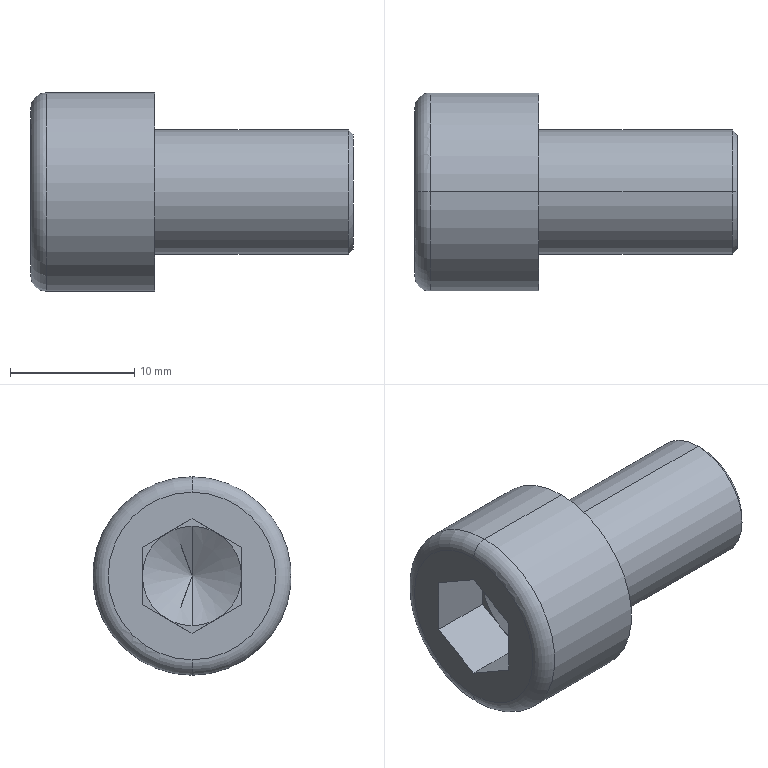Part | SolidWorks | features Fillet 2, RevCut 2, Boss 1, Chamfer 1, Cut 1, Extrusion 1, LPattern 1 | 1 solid | 25 faces | box 26 x 16 x 16 mm | volume 2933 mm3 | plane 15 | cone 4 | cylinder 4 | torus 2 | commonest cylinder face diameters 10 x2 16 x2
STEP:
#1=CARTESIAN_POINT('',(26.,0.,-4.6));
#2=VERTEX_POINT('',#1);
#3=CARTESIAN_POINT('',(26.,0.,4.6));
#4=VERTEX_POINT('',#3);
#5=CARTESIAN_POINT('',(26.,0.,0.));
#6=DIRECTION('',(1.,0.,0.));
#7=DIRECTION('',(0.,0.,-1.));
#8=AXIS2_PLACEMENT_3D('',#5,#6,#7);
#9=CIRCLE('',#8,4.6);
#10=EDGE_CURVE('',#2,#4,#9,.T.);
#11=ORIENTED_EDGE('',*,*,#10,.F.);
#12=CARTESIAN_POINT('',(25.6,0.,-5.));
#13=VERTEX_POINT('',#12);
#14=CARTESIAN_POINT('',(26.,0.,-4.6));
#15=DIRECTION('',(-0.7071,0.,-0.7071));
#16=VECTOR('',#15,1000.);
#17=LINE('',#14,#16);
#18=EDGE_CURVE('',#2,#13,#17,.T.);
#19=ORIENTED_EDGE('',*,*,#18,.T.);
#20=CARTESIAN_POINT('',(25.6,0.,5.));
#21=VERTEX_POINT('',#20);
#22=CARTESIAN_POINT('',(25.6,0.,0.));
#23=DIRECTION('',(-1.,0.,0.));
#24=DIRECTION('',(0.,0.,-1.));
#25=AXIS2_PLACEMENT_3D('',#22,#23,#24);
#26=CIRCLE('',#25,5.);
#27=EDGE_CURVE('',#21,#13,#26,.T.);
#28=ORIENTED_EDGE('',*,*,#27,.F.);
#29=CARTESIAN_POINT('',(26.,0.,4.6));
#30=DIRECTION('',(-0.7071,0.,0.7071));
#31=VECTOR('',#30,1000.);
#32=LINE('',#29,#31);
#33=EDGE_CURVE('',#4,#21,#32,.T.);
#34=ORIENTED_EDGE('',*,*,#33,.F.);
#35=EDGE_LOOP('',(#11,#19,#28,#34));
#36=FACE_OUTER_BOUND('',#35,.T.);
#37=CARTESIAN_POINT('',(26.,0.,0.));
#38=DIRECTION('',(-1.,0.,0.));
#39=DIRECTION('',(0.,0.,1.));
#40=AXIS2_PLACEMENT_3D('',#37,#38,#39);
#41=CONICAL_SURFACE('',#40,4.6,0.7854);
#42=ADVANCED_FACE('',(#36),#41,.T.);
#43=CARTESIAN_POINT('',(0.,0.,6.75));
#44=VERTEX_POINT('',#43);
#45=CARTESIAN_POINT('',(0.,0.,-6.75));
#46=VERTEX_POINT('',#45);
#47=CARTESIAN_POINT('',(0.,0.,0.));
#48=DIRECTION('',(-1.,0.,0.));
#49=DIRECTION('',(0.,0.,-1.));
#50=AXIS2_PLACEMENT_3D('',#47,#48,#49);
#51=CIRCLE('',#50,6.75);
#52=EDGE_CURVE('',#44,#46,#51,.T.);
#53=ORIENTED_EDGE('',*,*,#52,.F.);
#54=CARTESIAN_POINT('',(1.25,0.,8.));
#55=VERTEX_POINT('',#54);
#56=CARTESIAN_POINT('',(1.25,0.,6.75));
#57=DIRECTION('',(0.,1.,0.));
#58=DIRECTION('',(0.,0.,1.));
#59=AXIS2_PLACEMENT_3D('',#56,#57,#58);
#60=CIRCLE('',#59,1.25);
#61=EDGE_CURVE('',#44,#55,#60,.T.);
#62=ORIENTED_EDGE('',*,*,#61,.T.);
#63=CARTESIAN_POINT('',(1.25,0.,-8.));
#64=VERTEX_POINT('',#63);
#65=CARTESIAN_POINT('',(1.25,0.,0.));
#66=DIRECTION('',(1.,0.,0.));
#67=DIRECTION('',(0.,0.,-1.));
#68=AXIS2_PLACEMENT_3D('',#65,#66,#67);
#69=CIRCLE('',#68,8.);
#70=EDGE_CURVE('',#64,#55,#69,.T.);
#71=ORIENTED_EDGE('',*,*,#70,.F.);
#72=CARTESIAN_POINT('',(1.25,0.,-6.75));
#73=DIRECTION('',(0.,-1.,0.));
#74=DIRECTION('',(0.,0.,-1.));
#75=AXIS2_PLACEMENT_3D('',#72,#73,#74);
#76=CIRCLE('',#75,1.25);
#77=EDGE_CURVE('',#46,#64,#76,.T.);
#78=ORIENTED_EDGE('',*,*,#77,.F.);
#79=EDGE_LOOP('',(#53,#62,#71,#78));
#80=FACE_OUTER_BOUND('',#79,.T.);
#81=CARTESIAN_POINT('',(1.25,0.,0.));
#82=DIRECTION('',(1.,0.,0.));
#83=DIRECTION('',(0.,0.,-1.));
#84=AXIS2_PLACEMENT_3D('',#81,#82,#83);
#85=TOROIDAL_SURFACE('',#84,6.75,1.25);
#86=ADVANCED_FACE('',(#80),#85,.T.);
#87=CARTESIAN_POINT('',(7.309,0.,0.));
#88=VERTEX_POINT('',#87);
#89=CARTESIAN_POINT('',(5.,0.,4.));
#90=VERTEX_POINT('',#89);
#91=CARTESIAN_POINT('',(5.,0.,4.));
#92=DIRECTION('',(-0.5,0.,0.866));
#93=VECTOR('',#92,1000.);
#94=LINE('',#91,#93);
#95=EDGE_CURVE('',#88,#90,#94,.T.);
#96=ORIENTED_EDGE('',*,*,#95,.F.);
#97=CARTESIAN_POINT('',(5.,0.,-4.));
#98=VERTEX_POINT('',#97);
#99=CARTESIAN_POINT('',(5.,0.,-4.));
#100=DIRECTION('',(-0.5,0.,-0.866));
#101=VECTOR('',#100,1000.);
#102=LINE('',#99,#101);
#103=EDGE_CURVE('',#88,#98,#102,.T.);
#104=ORIENTED_EDGE('',*,*,#103,.T.);
#105=CARTESIAN_POINT('',(5.,-2.,-3.464));
#106=VERTEX_POINT('',#105);
#107=CARTESIAN_POINT('',(5.,0.,0.));
#108=DIRECTION('',(-1.,0.,0.));
#109=DIRECTION('',(0.,0.,-1.));
#110=AXIS2_PLACEMENT_3D('',#107,#108,#109);
#111=CIRCLE('',#110,4.);
#112=EDGE_CURVE('',#98,#106,#111,.T.);
#113=ORIENTED_EDGE('',*,*,#112,.T.);
#114=CARTESIAN_POINT('',(5.,-4.,0.));
#115=VERTEX_POINT('',#114);
#116=CARTESIAN_POINT('',(5.,0.,0.));
#117=DIRECTION('',(-1.,0.,0.));
#118=DIRECTION('',(0.,0.,-1.));
#119=AXIS2_PLACEMENT_3D('',#116,#117,#118);
#120=CIRCLE('',#119,4.);
#121=EDGE_CURVE('',#106,#115,#120,.T.);
#122=ORIENTED_EDGE('',*,*,#121,.T.);
#123=CARTESIAN_POINT('',(5.,-2.,3.464));
#124=VERTEX_POINT('',#123);
#125=CARTESIAN_POINT('',(5.,0.,0.));
#126=DIRECTION('',(-1.,0.,0.));
#127=DIRECTION('',(0.,0.,-1.));
#128=AXIS2_PLACEMENT_3D('',#125,#126,#127);
#129=CIRCLE('',#128,4.);
#130=EDGE_CURVE('',#115,#124,#129,.T.);
#131=ORIENTED_EDGE('',*,*,#130,.T.);
#132=CARTESIAN_POINT('',(5.,0.,0.));
#133=DIRECTION('',(-1.,0.,0.));
#134=DIRECTION('',(0.,0.,-1.));
#135=AXIS2_PLACEMENT_3D('',#132,#133,#134);
#136=CIRCLE('',#135,4.);
#137=EDGE_CURVE('',#124,#90,#136,.T.);
#138=ORIENTED_EDGE('',*,*,#137,.T.);
#139=EDGE_LOOP('',(#96,#104,#113,#122,#131,#138));
#140=FACE_OUTER_BOUND('',#139,.T.);
#141=CARTESIAN_POINT('',(5.,0.,0.));
#142=DIRECTION('',(-1.,0.,0.));
#143=DIRECTION('',(0.,0.,1.));
#144=AXIS2_PLACEMENT_3D('',#141,#142,#143);
#145=CONICAL_SURFACE('',#144,4.,1.047);
#146=ADVANCED_FACE('',(#140),#145,.F.);
#147=ORIENTED_EDGE('',*,*,#27,.T.);
#148=CARTESIAN_POINT('',(10.,0.,-5.));
#149=VERTEX_POINT('',#148);
#150=CARTESIAN_POINT('',(26.,0.,-5.));
#151=DIRECTION('',(-1.,0.,0.));
#152=VECTOR('',#151,1000.);
#153=LINE('',#150,#152);
#154=EDGE_CURVE('',#13,#149,#153,.T.);
#155=ORIENTED_EDGE('',*,*,#154,.T.);
#156=CARTESIAN_POINT('',(10.,0.,5.));
#157=VERTEX_POINT('',#156);
#158=CARTESIAN_POINT('',(10.,0.,0.));
#159=DIRECTION('',(1.,0.,0.));
#160=DIRECTION('',(0.,0.,-1.));
#161=AXIS2_PLACEMENT_3D('',#158,#159,#160);
#162=CIRCLE('',#161,5.);
#163=EDGE_CURVE('',#149,#157,#162,.T.);
#164=ORIENTED_EDGE('',*,*,#163,.T.);
#165=CARTESIAN_POINT('',(26.,0.,5.));
#166=DIRECTION('',(-1.,0.,0.));
#167=VECTOR('',#166,1000.);
#168=LINE('',#165,#167);
#169=EDGE_CURVE('',#21,#157,#168,.T.);
#170=ORIENTED_EDGE('',*,*,#169,.F.);
#171=EDGE_LOOP('',(#147,#155,#164,#170));
#172=FACE_OUTER_BOUND('',#171,.T.);
#173=CARTESIAN_POINT('',(26.,0.,0.));
#174=DIRECTION('',(-1.,0.,0.));
#175=DIRECTION('',(0.,0.,1.));
#176=AXIS2_PLACEMENT_3D('',#173,#174,#175);
#177=CYLINDRICAL_SURFACE('',#176,5.);
#178=ADVANCED_FACE('',(#172),#177,.T.);
#179=CARTESIAN_POINT('',(10.,0.,-8.));
#180=VERTEX_POINT('',#179);
#181=CARTESIAN_POINT('',(10.,0.,8.));
#182=VERTEX_POINT('',#181);
#183=CARTESIAN_POINT('',(10.,0.,0.));
#184=DIRECTION('',(1.,0.,0.));
#185=DIRECTION('',(0.,0.,-1.));
#186=AXIS2_PLACEMENT_3D('',#183,#184,#185);
#187=CIRCLE('',#186,8.);
#188=EDGE_CURVE('',#180,#182,#187,.T.);
#189=ORIENTED_EDGE('',*,*,#188,.F.);
#190=CARTESIAN_POINT('',(10.,0.,-8.));
#191=DIRECTION('',(-1.,0.,0.));
#192=VECTOR('',#191,1000.);
#193=LINE('',#190,#192);
#194=EDGE_CURVE('',#180,#64,#193,.T.);
#195=ORIENTED_EDGE('',*,*,#194,.T.);
#196=ORIENTED_EDGE('',*,*,#70,.T.);
#197=CARTESIAN_POINT('',(10.,0.,8.));
#198=DIRECTION('',(-1.,0.,0.));
#199=VECTOR('',#198,1000.);
#200=LINE('',#197,#199);
#201=EDGE_CURVE('',#182,#55,#200,.T.);
#202=ORIENTED_EDGE('',*,*,#201,.F.);
#203=EDGE_LOOP('',(#189,#195,#196,#202));
#204=FACE_OUTER_BOUND('',#203,.T.);
#205=CARTESIAN_POINT('',(10.,0.,0.));
#206=DIRECTION('',(-1.,0.,0.));
#207=DIRECTION('',(0.,0.,1.));
#208=AXIS2_PLACEMENT_3D('',#205,#206,#207);
#209=CYLINDRICAL_SURFACE('',#208,8.);
#210=ADVANCED_FACE('',(#204),#209,.T.);
#211=ORIENTED_EDGE('',*,*,#121,.F.);
#212=CARTESIAN_POINT('',(5.,-4.,-2.309));
#213=VERTEX_POINT('',#212);
#214=CARTESIAN_POINT('',(5.,-4.,-2.309));
#215=DIRECTION('',(0.,0.866,-0.5));
#216=VECTOR('',#215,1000.);
#217=LINE('',#214,#216);
#218=EDGE_CURVE('',#213,#106,#217,.T.);
#219=ORIENTED_EDGE('',*,*,#218,.F.);
#220=CARTESIAN_POINT('',(5.,-4.,2.309));
#221=DIRECTION('',(0.,0.,-1.));
#222=VECTOR('',#221,1000.);
#223=LINE('',#220,#222);
#224=EDGE_CURVE('',#115,#213,#223,.T.);
#225=ORIENTED_EDGE('',*,*,#224,.F.);
#226=EDGE_LOOP('',(#211,#219,#225));
#227=FACE_OUTER_BOUND('',#226,.T.);
#228=CARTESIAN_POINT('',(5.,0.,-4.619));
#229=DIRECTION('',(1.,0.,0.));
#230=DIRECTION('',(0.,0.,-1.));
#231=AXIS2_PLACEMENT_3D('',#228,#229,#230);
#232=PLANE('',#231);
#233=ADVANCED_FACE('',(#227),#232,.F.);
#234=ORIENTED_EDGE('',*,*,#130,.F.);
#235=CARTESIAN_POINT('',(5.,-4.,2.309));
#236=VERTEX_POINT('',#235);
#237=CARTESIAN_POINT('',(5.,-4.,2.309));
#238=DIRECTION('',(0.,0.,-1.));
#239=VECTOR('',#238,1000.);
#240=LINE('',#237,#239);
#241=EDGE_CURVE('',#236,#115,#240,.T.);
#242=ORIENTED_EDGE('',*,*,#241,.F.);
#243=CARTESIAN_POINT('',(5.,0.,4.619));
#244=DIRECTION('',(0.,-0.866,-0.5));
#245=VECTOR('',#244,1000.);
#246=LINE('',#243,#245);
#247=EDGE_CURVE('',#124,#236,#246,.T.);
#248=ORIENTED_EDGE('',*,*,#247,.F.);
#249=EDGE_LOOP('',(#234,#242,#248));
#250=FACE_OUTER_BOUND('',#249,.T.);
#251=CARTESIAN_POINT('',(5.,0.,-4.619));
#252=DIRECTION('',(1.,0.,0.));
#253=DIRECTION('',(0.,0.,-1.));
#254=AXIS2_PLACEMENT_3D('',#251,#252,#253);
#255=PLANE('',#254);
#256=ADVANCED_FACE('',(#250),#255,.F.);
#257=ORIENTED_EDGE('',*,*,#137,.F.);
#258=CARTESIAN_POINT('',(5.,0.,4.619));
#259=VERTEX_POINT('',#258);
#260=CARTESIAN_POINT('',(5.,0.,4.619));
#261=DIRECTION('',(0.,-0.866,-0.5));
#262=VECTOR('',#261,1000.);
#263=LINE('',#260,#262);
#264=EDGE_CURVE('',#259,#124,#263,.T.);
#265=ORIENTED_EDGE('',*,*,#264,.F.);
#266=CARTESIAN_POINT('',(5.,2.,3.464));
#267=VERTEX_POINT('',#266);
#268=CARTESIAN_POINT('',(5.,4.,2.309));
#269=DIRECTION('',(0.,-0.866,0.5));
#270=VECTOR('',#269,1000.);
#271=LINE('',#268,#270);
#272=EDGE_CURVE('',#267,#259,#271,.T.);
#273=ORIENTED_EDGE('',*,*,#272,.F.);
#274=CARTESIAN_POINT('',(5.,0.,0.));
#275=DIRECTION('',(-1.,0.,0.));
#276=DIRECTION('',(0.,0.,-1.));
#277=AXIS2_PLACEMENT_3D('',#274,#275,#276);
#278=CIRCLE('',#277,4.);
#279=EDGE_CURVE('',#90,#267,#278,.T.);
#280=ORIENTED_EDGE('',*,*,#279,.F.);
#281=EDGE_LOOP('',(#257,#265,#273,#280));
#282=FACE_OUTER_BOUND('',#281,.T.);
#283=CARTESIAN_POINT('',(5.,0.,-4.619));
#284=DIRECTION('',(1.,0.,0.));
#285=DIRECTION('',(0.,0.,-1.));
#286=AXIS2_PLACEMENT_3D('',#283,#284,#285);
#287=PLANE('',#286);
#288=ADVANCED_FACE('',(#282),#287,.F.);
#289=CARTESIAN_POINT('',(5.,4.,0.));
#290=VERTEX_POINT('',#289);
#291=CARTESIAN_POINT('',(5.,0.,0.));
#292=DIRECTION('',(-1.,0.,0.));
#293=DIRECTION('',(0.,0.,-1.));
#294=AXIS2_PLACEMENT_3D('',#291,#292,#293);
#295=CIRCLE('',#294,4.);
#296=EDGE_CURVE('',#267,#290,#295,.T.);
#297=ORIENTED_EDGE('',*,*,#296,.F.);
#298=CARTESIAN_POINT('',(5.,4.,2.309));
#299=VERTEX_POINT('',#298);
#300=CARTESIAN_POINT('',(5.,4.,2.309));
#301=DIRECTION('',(0.,-0.866,0.5));
#302=VECTOR('',#301,1000.);
#303=LINE('',#300,#302);
#304=EDGE_CURVE('',#299,#267,#303,.T.);
#305=ORIENTED_EDGE('',*,*,#304,.F.);
#306=CARTESIAN_POINT('',(5.,4.,-2.309));
#307=DIRECTION('',(0.,0.,1.));
#308=VECTOR('',#307,1000.);
#309=LINE('',#306,#308);
#310=EDGE_CURVE('',#290,#299,#309,.T.);
#311=ORIENTED_EDGE('',*,*,#310,.F.);
#312=EDGE_LOOP('',(#297,#305,#311));
#313=FACE_OUTER_BOUND('',#312,.T.);
#314=CARTESIAN_POINT('',(5.,0.,-4.619));
#315=DIRECTION('',(1.,0.,0.));
#316=DIRECTION('',(0.,0.,-1.));
#317=AXIS2_PLACEMENT_3D('',#314,#315,#316);
#318=PLANE('',#317);
#319=ADVANCED_FACE('',(#313),#318,.F.);
#320=CARTESIAN_POINT('',(5.,2.,-3.464));
#321=VERTEX_POINT('',#320);
#322=CARTESIAN_POINT('',(5.,0.,0.));
#323=DIRECTION('',(1.,0.,0.));
#324=DIRECTION('',(0.,0.,-1.));
#325=AXIS2_PLACEMENT_3D('',#322,#323,#324);
#326=CIRCLE('',#325,4.);
#327=EDGE_CURVE('',#321,#290,#326,.T.);
#328=ORIENTED_EDGE('',*,*,#327,.T.);
#329=CARTESIAN_POINT('',(5.,4.,-2.309));
#330=VERTEX_POINT('',#329);
#331=CARTESIAN_POINT('',(5.,4.,-2.309));
#332=DIRECTION('',(0.,0.,1.));
#333=VECTOR('',#332,1000.);
#334=LINE('',#331,#333);
#335=EDGE_CURVE('',#330,#290,#334,.T.);
#336=ORIENTED_EDGE('',*,*,#335,.F.);
#337=CARTESIAN_POINT('',(5.,0.,-4.619));
#338=DIRECTION('',(0.,0.866,0.5));
#339=VECTOR('',#338,1000.);
#340=LINE('',#337,#339);
#341=EDGE_CURVE('',#321,#330,#340,.T.);
#342=ORIENTED_EDGE('',*,*,#341,.F.);
#343=EDGE_LOOP('',(#328,#336,#342));
#344=FACE_OUTER_BOUND('',#343,.T.);
#345=CARTESIAN_POINT('',(5.,0.,-4.619));
#346=DIRECTION('',(1.,0.,0.));
#347=DIRECTION('',(0.,0.,-1.));
#348=AXIS2_PLACEMENT_3D('',#345,#346,#347);
#349=PLANE('',#348);
#350=ADVANCED_FACE('',(#344),#349,.F.);
#351=CARTESIAN_POINT('',(5.,0.,0.));
#352=DIRECTION('',(-1.,0.,0.));
#353=DIRECTION('',(0.,0.,-1.));
#354=AXIS2_PLACEMENT_3D('',#351,#352,#353);
#355=CIRCLE('',#354,4.);
#356=EDGE_CURVE('',#321,#98,#355,.T.);
#357=ORIENTED_EDGE('',*,*,#356,.F.);
#358=CARTESIAN_POINT('',(5.,0.,-4.619));
#359=VERTEX_POINT('',#358);
#360=CARTESIAN_POINT('',(5.,0.,-4.619));
#361=DIRECTION('',(0.,0.866,0.5));
#362=VECTOR('',#361,1000.);
#363=LINE('',#360,#362);
#364=EDGE_CURVE('',#359,#321,#363,.T.);
#365=ORIENTED_EDGE('',*,*,#364,.F.);
#366=CARTESIAN_POINT('',(5.,-4.,-2.309));
#367=DIRECTION('',(0.,0.866,-0.5));
#368=VECTOR('',#367,1000.);
#369=LINE('',#366,#368);
#370=EDGE_CURVE('',#106,#359,#369,.T.);
#371=ORIENTED_EDGE('',*,*,#370,.F.);
#372=ORIENTED_EDGE('',*,*,#112,.F.);
#373=EDGE_LOOP('',(#357,#365,#371,#372));
#374=FACE_OUTER_BOUND('',#373,.T.);
#375=CARTESIAN_POINT('',(5.,0.,-4.619));
#376=DIRECTION('',(1.,0.,0.));
#377=DIRECTION('',(0.,0.,-1.));
#378=AXIS2_PLACEMENT_3D('',#375,#376,#377);
#379=PLANE('',#378);
#380=ADVANCED_FACE('',(#374),#379,.F.);
#381=CARTESIAN_POINT('',(0.,0.,0.));
#382=DIRECTION('',(-1.,0.,0.));
#383=DIRECTION('',(0.,0.,-1.));
#384=AXIS2_PLACEMENT_3D('',#381,#382,#383);
#385=CIRCLE('',#384,6.75);
#386=EDGE_CURVE('',#46,#44,#385,.T.);
#387=ORIENTED_EDGE('',*,*,#386,.T.);
#388=ORIENTED_EDGE('',*,*,#52,.T.);
#389=EDGE_LOOP('',(#387,#388));
#390=FACE_OUTER_BOUND('',#389,.T.);
#391=CARTESIAN_POINT('',(0.,-4.,-2.309));
#392=VERTEX_POINT('',#391);
#393=CARTESIAN_POINT('',(0.,0.,-4.619));
#394=VERTEX_POINT('',#393);
#395=CARTESIAN_POINT('',(0.,-4.,-2.309));
#396=DIRECTION('',(0.,0.866,-0.5));
#397=VECTOR('',#396,1000.);
#398=LINE('',#395,#397);
#399=EDGE_CURVE('',#392,#394,#398,.T.);
#400=ORIENTED_EDGE('',*,*,#399,.T.);
#401=CARTESIAN_POINT('',(0.,4.,-2.309));
#402=VERTEX_POINT('',#401);
#403=CARTESIAN_POINT('',(0.,0.,-4.619));
#404=DIRECTION('',(0.,0.866,0.5));
#405=VECTOR('',#404,1000.);
#406=LINE('',#403,#405);
#407=EDGE_CURVE('',#394,#402,#406,.T.);
#408=ORIENTED_EDGE('',*,*,#407,.T.);
#409=CARTESIAN_POINT('',(0.,4.,2.309));
#410=VERTEX_POINT('',#409);
#411=CARTESIAN_POINT('',(0.,4.,-2.309));
#412=DIRECTION('',(0.,0.,1.));
#413=VECTOR('',#412,1000.);
#414=LINE('',#411,#413);
#415=EDGE_CURVE('',#402,#410,#414,.T.);
#416=ORIENTED_EDGE('',*,*,#415,.T.);
#417=CARTESIAN_POINT('',(0.,0.,4.619));
#418=VERTEX_POINT('',#417);
#419=CARTESIAN_POINT('',(0.,4.,2.309));
#420=DIRECTION('',(0.,-0.866,0.5));
#421=VECTOR('',#420,1000.);
#422=LINE('',#419,#421);
#423=EDGE_CURVE('',#410,#418,#422,.T.);
#424=ORIENTED_EDGE('',*,*,#423,.T.);
#425=CARTESIAN_POINT('',(0.,-4.,2.309));
#426=VERTEX_POINT('',#425);
#427=CARTESIAN_POINT('',(0.,0.,4.619));
#428=DIRECTION('',(0.,-0.866,-0.5));
#429=VECTOR('',#428,1000.);
#430=LINE('',#427,#429);
#431=EDGE_CURVE('',#418,#426,#430,.T.);
#432=ORIENTED_EDGE('',*,*,#431,.T.);
#433=CARTESIAN_POINT('',(0.,-4.,2.309));
#434=DIRECTION('',(0.,0.,-1.));
#435=VECTOR('',#434,1000.);
#436=LINE('',#433,#435);
#437=EDGE_CURVE('',#426,#392,#436,.T.);
#438=ORIENTED_EDGE('',*,*,#437,.T.);
#439=EDGE_LOOP('',(#400,#408,#416,#424,#432,#438));
#440=FACE_BOUND('',#439,.T.);
#441=CARTESIAN_POINT('',(0.,0.,0.));
#442=DIRECTION('',(1.,0.,0.));
#443=DIRECTION('',(0.,0.,-1.));
#444=AXIS2_PLACEMENT_3D('',#441,#442,#443);
#445=PLANE('',#444);
#446=ADVANCED_FACE('',(#390,#440),#445,.F.);
#447=CARTESIAN_POINT('',(10.,0.,0.));
#448=DIRECTION('',(1.,0.,0.));
#449=DIRECTION('',(0.,0.,-1.));
#450=AXIS2_PLACEMENT_3D('',#447,#448,#449);
#451=CIRCLE('',#450,8.);
#452=EDGE_CURVE('',#182,#180,#451,.T.);
#453=ORIENTED_EDGE('',*,*,#452,.T.);
#454=ORIENTED_EDGE('',*,*,#188,.T.);
#455=EDGE_LOOP('',(#453,#454));
#456=FACE_OUTER_BOUND('',#455,.T.);
#457=CARTESIAN_POINT('',(10.,0.,0.));
#458=DIRECTION('',(1.,0.,0.));
#459=DIRECTION('',(0.,0.,-1.));
#460=AXIS2_PLACEMENT_3D('',#457,#458,#459);
#461=CIRCLE('',#460,5.);
#462=EDGE_CURVE('',#157,#149,#461,.T.);
#463=ORIENTED_EDGE('',*,*,#462,.F.);
#464=ORIENTED_EDGE('',*,*,#163,.F.);
#465=EDGE_LOOP('',(#463,#464));
#466=FACE_BOUND('',#465,.T.);
#467=CARTESIAN_POINT('',(10.,0.,0.));
#468=DIRECTION('',(1.,0.,0.));
#469=DIRECTION('',(0.,0.,-1.));
#470=AXIS2_PLACEMENT_3D('',#467,#468,#469);
#471=PLANE('',#470);
#472=ADVANCED_FACE('',(#456,#466),#471,.T.);
#473=ORIENTED_EDGE('',*,*,#194,.F.);
#474=ORIENTED_EDGE('',*,*,#452,.F.);
#475=ORIENTED_EDGE('',*,*,#201,.T.);
#476=CARTESIAN_POINT('',(1.25,0.,0.));
#477=DIRECTION('',(1.,0.,0.));
#478=DIRECTION('',(0.,0.,-1.));
#479=AXIS2_PLACEMENT_3D('',#476,#477,#478);
#480=CIRCLE('',#479,8.);
#481=EDGE_CURVE('',#55,#64,#480,.T.);
#482=ORIENTED_EDGE('',*,*,#481,.T.);
#483=EDGE_LOOP('',(#473,#474,#475,#482));
#484=FACE_OUTER_BOUND('',#483,.T.);
#485=CARTESIAN_POINT('',(10.,0.,0.));
#486=DIRECTION('',(-1.,0.,0.));
#487=DIRECTION('',(0.,0.,1.));
#488=AXIS2_PLACEMENT_3D('',#485,#486,#487);
#489=CYLINDRICAL_SURFACE('',#488,8.);
#490=ADVANCED_FACE('',(#484),#489,.T.);
#491=ORIENTED_EDGE('',*,*,#154,.F.);
#492=CARTESIAN_POINT('',(25.6,0.,0.));
#493=DIRECTION('',(-1.,0.,0.));
#494=DIRECTION('',(0.,0.,-1.));
#495=AXIS2_PLACEMENT_3D('',#492,#493,#494);
#496=CIRCLE('',#495,5.);
#497=EDGE_CURVE('',#13,#21,#496,.T.);
#498=ORIENTED_EDGE('',*,*,#497,.T.);
#499=ORIENTED_EDGE('',*,*,#169,.T.);
#500=ORIENTED_EDGE('',*,*,#462,.T.);
#501=EDGE_LOOP('',(#491,#498,#499,#500));
#502=FACE_OUTER_BOUND('',#501,.T.);
#503=CARTESIAN_POINT('',(26.,0.,0.));
#504=DIRECTION('',(-1.,0.,0.));
#505=DIRECTION('',(0.,0.,1.));
#506=AXIS2_PLACEMENT_3D('',#503,#504,#505);
#507=CYLINDRICAL_SURFACE('',#506,5.);
#508=ADVANCED_FACE('',(#502),#507,.T.);
#509=CARTESIAN_POINT('',(26.,0.,0.));
#510=DIRECTION('',(1.,0.,0.));
#511=DIRECTION('',(0.,0.,-1.));
#512=AXIS2_PLACEMENT_3D('',#509,#510,#511);
#513=CIRCLE('',#512,4.6);
#514=EDGE_CURVE('',#4,#2,#513,.T.);
#515=ORIENTED_EDGE('',*,*,#514,.T.);
#516=ORIENTED_EDGE('',*,*,#10,.T.);
#517=EDGE_LOOP('',(#515,#516));
#518=FACE_OUTER_BOUND('',#517,.T.);
#519=CARTESIAN_POINT('',(26.,0.,0.));
#520=DIRECTION('',(1.,0.,0.));
#521=DIRECTION('',(0.,0.,-1.));
#522=AXIS2_PLACEMENT_3D('',#519,#520,#521);
#523=PLANE('',#522);
#524=ADVANCED_FACE('',(#518),#523,.T.);
#525=ORIENTED_EDGE('',*,*,#399,.F.);
#526=CARTESIAN_POINT('',(5.,-4.,-2.309));
#527=DIRECTION('',(-1.,0.,0.));
#528=VECTOR('',#527,1000.);
#529=LINE('',#526,#528);
#530=EDGE_CURVE('',#213,#392,#529,.T.);
#531=ORIENTED_EDGE('',*,*,#530,.F.);
#532=ORIENTED_EDGE('',*,*,#218,.T.);
#533=ORIENTED_EDGE('',*,*,#370,.T.);
#534=CARTESIAN_POINT('',(5.,0.,-4.619));
#535=DIRECTION('',(-1.,0.,0.));
#536=VECTOR('',#535,1000.);
#537=LINE('',#534,#536);
#538=EDGE_CURVE('',#359,#394,#537,.T.);
#539=ORIENTED_EDGE('',*,*,#538,.T.);
#540=EDGE_LOOP('',(#525,#531,#532,#533,#539));
#541=FACE_OUTER_BOUND('',#540,.T.);
#542=CARTESIAN_POINT('',(5.,-4.,-2.309));
#543=DIRECTION('',(0.,0.5,0.866));
#544=DIRECTION('',(0.,-0.866,0.5));
#545=AXIS2_PLACEMENT_3D('',#542,#543,#544);
#546=PLANE('',#545);
#547=ADVANCED_FACE('',(#541),#546,.T.);
#548=ORIENTED_EDGE('',*,*,#407,.F.);
#549=ORIENTED_EDGE('',*,*,#538,.F.);
#550=ORIENTED_EDGE('',*,*,#364,.T.);
#551=ORIENTED_EDGE('',*,*,#341,.T.);
#552=CARTESIAN_POINT('',(5.,4.,-2.309));
#553=DIRECTION('',(-1.,0.,0.));
#554=VECTOR('',#553,1000.);
#555=LINE('',#552,#554);
#556=EDGE_CURVE('',#330,#402,#555,.T.);
#557=ORIENTED_EDGE('',*,*,#556,.T.);
#558=EDGE_LOOP('',(#548,#549,#550,#551,#557));
#559=FACE_OUTER_BOUND('',#558,.T.);
#560=CARTESIAN_POINT('',(5.,0.,-4.619));
#561=DIRECTION('',(0.,-0.5,0.866));
#562=DIRECTION('',(0.,-0.866,-0.5));
#563=AXIS2_PLACEMENT_3D('',#560,#561,#562);
#564=PLANE('',#563);
#565=ADVANCED_FACE('',(#559),#564,.T.);
#566=ORIENTED_EDGE('',*,*,#415,.F.);
#567=ORIENTED_EDGE('',*,*,#556,.F.);
#568=ORIENTED_EDGE('',*,*,#335,.T.);
#569=ORIENTED_EDGE('',*,*,#310,.T.);
#570=CARTESIAN_POINT('',(5.,4.,2.309));
#571=DIRECTION('',(-1.,0.,0.));
#572=VECTOR('',#571,1000.);
#573=LINE('',#570,#572);
#574=EDGE_CURVE('',#299,#410,#573,.T.);
#575=ORIENTED_EDGE('',*,*,#574,.T.);
#576=EDGE_LOOP('',(#566,#567,#568,#569,#575));
#577=FACE_OUTER_BOUND('',#576,.T.);
#578=CARTESIAN_POINT('',(5.,4.,-2.309));
#579=DIRECTION('',(0.,-1.,0.));
#580=DIRECTION('',(0.,0.,-1.));
#581=AXIS2_PLACEMENT_3D('',#578,#579,#580);
#582=PLANE('',#581);
#583=ADVANCED_FACE('',(#577),#582,.T.);
#584=ORIENTED_EDGE('',*,*,#423,.F.);
#585=ORIENTED_EDGE('',*,*,#574,.F.);
#586=ORIENTED_EDGE('',*,*,#304,.T.);
#587=ORIENTED_EDGE('',*,*,#272,.T.);
#588=CARTESIAN_POINT('',(5.,0.,4.619));
#589=DIRECTION('',(-1.,0.,0.));
#590=VECTOR('',#589,1000.);
#591=LINE('',#588,#590);
#592=EDGE_CURVE('',#259,#418,#591,.T.);
#593=ORIENTED_EDGE('',*,*,#592,.T.);
#594=EDGE_LOOP('',(#584,#585,#586,#587,#593));
#595=FACE_OUTER_BOUND('',#594,.T.);
#596=CARTESIAN_POINT('',(5.,4.,2.309));
#597=DIRECTION('',(0.,-0.5,-0.866));
#598=DIRECTION('',(0.,0.866,-0.5));
#599=AXIS2_PLACEMENT_3D('',#596,#597,#598);
#600=PLANE('',#599);
#601=ADVANCED_FACE('',(#595),#600,.T.);
#602=ORIENTED_EDGE('',*,*,#431,.F.);
#603=ORIENTED_EDGE('',*,*,#592,.F.);
#604=ORIENTED_EDGE('',*,*,#264,.T.);
#605=ORIENTED_EDGE('',*,*,#247,.T.);
#606=CARTESIAN_POINT('',(5.,-4.,2.309));
#607=DIRECTION('',(-1.,0.,0.));
#608=VECTOR('',#607,1000.);
#609=LINE('',#606,#608);
#610=EDGE_CURVE('',#236,#426,#609,.T.);
#611=ORIENTED_EDGE('',*,*,#610,.T.);
#612=EDGE_LOOP('',(#602,#603,#604,#605,#611));
#613=FACE_OUTER_BOUND('',#612,.T.);
#614=CARTESIAN_POINT('',(5.,0.,4.619));
#615=DIRECTION('',(0.,0.5,-0.866));
#616=DIRECTION('',(0.,0.866,0.5));
#617=AXIS2_PLACEMENT_3D('',#614,#615,#616);
#618=PLANE('',#617);
#619=ADVANCED_FACE('',(#613),#618,.T.);
#620=ORIENTED_EDGE('',*,*,#437,.F.);
#621=ORIENTED_EDGE('',*,*,#610,.F.);
#622=ORIENTED_EDGE('',*,*,#241,.T.);
#623=ORIENTED_EDGE('',*,*,#224,.T.);
#624=ORIENTED_EDGE('',*,*,#530,.T.);
#625=EDGE_LOOP('',(#620,#621,#622,#623,#624));
#626=FACE_OUTER_BOUND('',#625,.T.);
#627=CARTESIAN_POINT('',(5.,-4.,2.309));
#628=DIRECTION('',(0.,1.,0.));
#629=DIRECTION('',(0.,0.,1.));
#630=AXIS2_PLACEMENT_3D('',#627,#628,#629);
#631=PLANE('',#630);
#632=ADVANCED_FACE('',(#626),#631,.T.);
#633=ORIENTED_EDGE('',*,*,#103,.F.);
#634=ORIENTED_EDGE('',*,*,#95,.T.);
#635=ORIENTED_EDGE('',*,*,#279,.T.);
#636=ORIENTED_EDGE('',*,*,#296,.T.);
#637=ORIENTED_EDGE('',*,*,#327,.F.);
#638=ORIENTED_EDGE('',*,*,#356,.T.);
#639=EDGE_LOOP('',(#633,#634,#635,#636,#637,#638));
#640=FACE_OUTER_BOUND('',#639,.T.);
#641=CARTESIAN_POINT('',(5.,0.,0.));
#642=DIRECTION('',(-1.,0.,0.));
#643=DIRECTION('',(0.,0.,1.));
#644=AXIS2_PLACEMENT_3D('',#641,#642,#643);
#645=CONICAL_SURFACE('',#644,4.,1.047);
#646=ADVANCED_FACE('',(#640),#645,.F.);
#647=ORIENTED_EDGE('',*,*,#61,.F.);
#648=ORIENTED_EDGE('',*,*,#386,.F.);
#649=ORIENTED_EDGE('',*,*,#77,.T.);
#650=ORIENTED_EDGE('',*,*,#481,.F.);
#651=EDGE_LOOP('',(#647,#648,#649,#650));
#652=FACE_OUTER_BOUND('',#651,.T.);
#653=CARTESIAN_POINT('',(1.25,0.,0.));
#654=DIRECTION('',(1.,0.,0.));
#655=DIRECTION('',(0.,0.,-1.));
#656=AXIS2_PLACEMENT_3D('',#653,#654,#655);
#657=TOROIDAL_SURFACE('',#656,6.75,1.25);
#658=ADVANCED_FACE('',(#652),#657,.T.);
#659=ORIENTED_EDGE('',*,*,#18,.F.);
#660=ORIENTED_EDGE('',*,*,#514,.F.);
#661=ORIENTED_EDGE('',*,*,#33,.T.);
#662=ORIENTED_EDGE('',*,*,#497,.F.);
#663=EDGE_LOOP('',(#659,#660,#661,#662));
#664=FACE_OUTER_BOUND('',#663,.T.);
#665=CARTESIAN_POINT('',(26.,0.,0.));
#666=DIRECTION('',(-1.,0.,0.));
#667=DIRECTION('',(0.,0.,1.));
#668=AXIS2_PLACEMENT_3D('',#665,#666,#667);
#669=CONICAL_SURFACE('',#668,4.6,0.7854);
#670=ADVANCED_FACE('',(#664),#669,.T.);
#671=CLOSED_SHELL('',(#42,#86,#146,#178,#210,#233,#256,#288,#319,#350,#380,#446,#472,#490,#508,#524,#547,#565,#583,#601,#619,#632,#646,#658,#670));
#672=MANIFOLD_SOLID_BREP('',#671);
#673=CARTESIAN_POINT('',(0.,0.,0.));
#674=DIRECTION('',(0.,0.,1.));
#675=DIRECTION('',(1.,0.,0.));
#676=AXIS2_PLACEMENT_3D('',#673,#674,#675);
#677=(LENGTH_UNIT()NAMED_UNIT(*)SI_UNIT(.MILLI.,.METRE.));
#678=UNCERTAINTY_MEASURE_WITH_UNIT(LENGTH_MEASURE(0.00001),#677,'','');
#679=(NAMED_UNIT(*)PLANE_ANGLE_UNIT()SI_UNIT($,.RADIAN.));
#680=(NAMED_UNIT(*)SI_UNIT($,.STERADIAN.)SOLID_ANGLE_UNIT());
#681=(GEOMETRIC_REPRESENTATION_CONTEXT(3)GLOBAL_UNCERTAINTY_ASSIGNED_CONTEXT((#678))GLOBAL_UNIT_ASSIGNED_CONTEXT((#677,#679,#680))REPRESENTATION_CONTEXT('',''));
#682=ADVANCED_BREP_SHAPE_REPRESENTATION('',(#672,#676),#681);